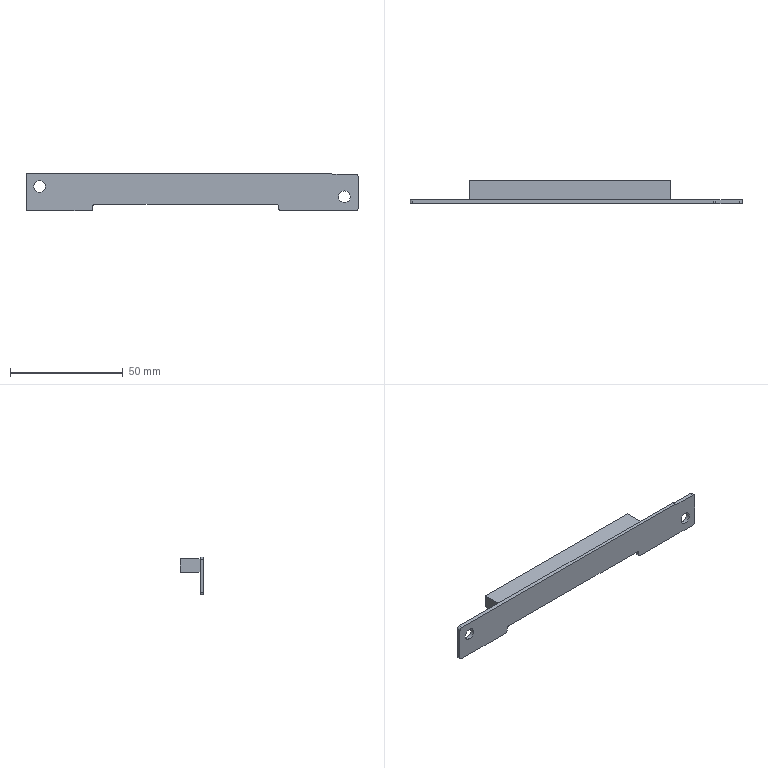Part | SolidWorks | features ICE 3, Extrusion 1, MoveFace 1 | 1 solid | 41 faces | box 147 x 10.5 x 16.8 mm | volume 7195 mm3 | plane 26 | cylinder 15 | commonest cylinder face diameters 2 x11 5.207 x4